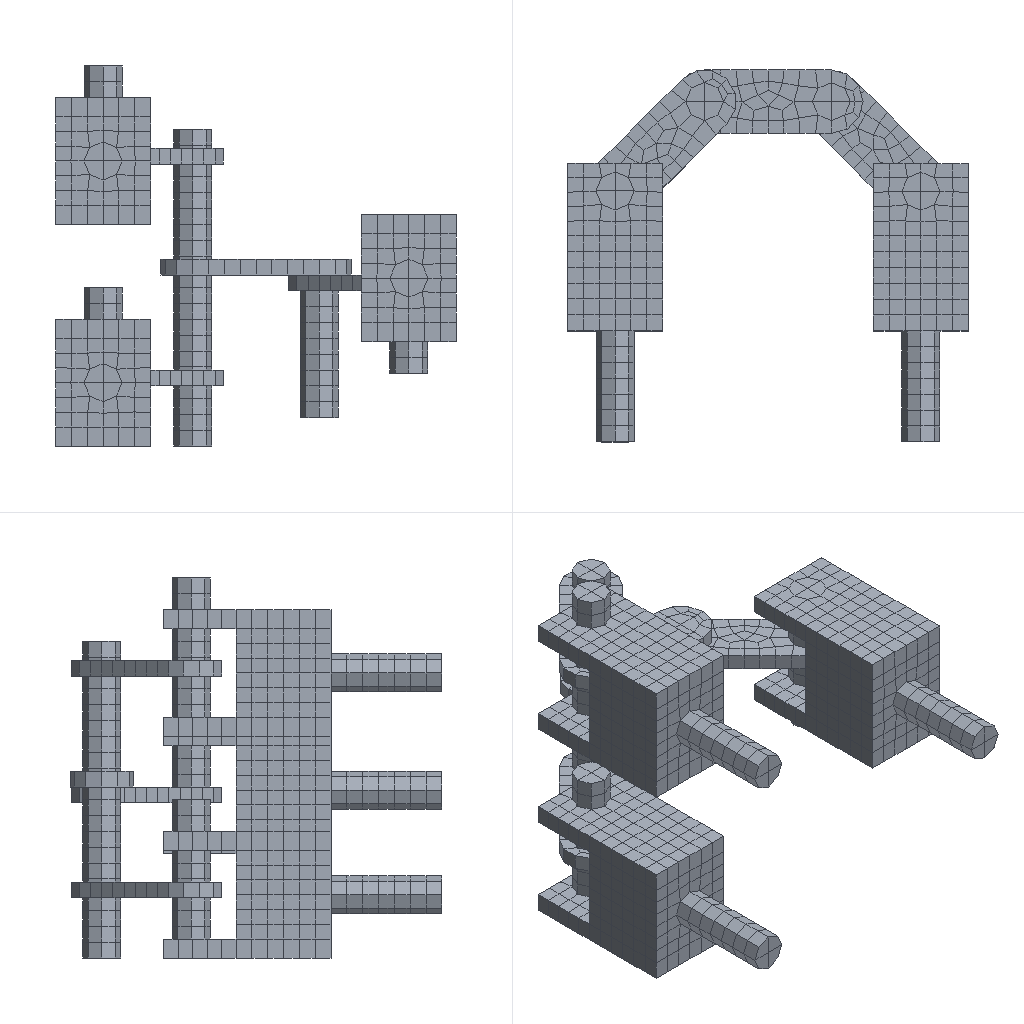Simulation study | abaqus
Set-up summary:
category,name,step,type,value,unit,region
solver,abaqus
solver,version,,,Abaqus/Explicit 2020
units,not stated in the deck,,not stated
analysis,deck,,transient,transient
load_step,Step-1,Step-1,transient
load_step,requested,,,1
mesh,nodes,,,3136
mesh,elements,,,1496
element_type,C3D8R,,solid,1496
load,load commands in deck,,count,1
bc,support commands in deck,,count,10
material,MATERIAL-1,,in results
check,setup vs results,,match,"per instance, exact: element labels, types and connectivity; labels of the nodes the elements use; coordinates of those nodes at SINGLE_PRECISION in 12 of 15 instance(s)"
Abaqus input file, long lists of numbers shortened:
*Heading
** Job name: Job-1 Model name: Model-1
** Generated by: Abaqus/CAE 2020
*Preprint, echo=NO, model=NO, history=NO, contact=NO
**
** PARTS
**
*Part, name=Part-1
*End Part
**
*Part, name=Part-2
*End Part
**
*Part, name=Part-3
*End Part
**
*Part, name=Part-4
*End Part
**
**
** ASSEMBLY
**
*Assembly, name=Assembly
**
*Instance, name=Part-1-1, part=Part-1
*Node
      1,          15.,          15.,           0.
      2,         -15.,          15.,           0.
** (568 more lines like these left out)
*Element, type=C3D8R
 1, 205,  46,  45, 200, 216,  57,  58, 211
 2, 204,  33,  32, 197, 215,  70,  71, 208
** (314 more lines like these left out)
*Nset, nset=Set-1, generate
   1,  570,    1
*Elset, elset=Set-1, generate
   1,  316,    1
** Section: Section-1
*Solid Section, elset=Set-1, material=Material-1
,
*End Instance
**
*Instance, name=Part-2-1, part=Part-2
          0.,         29.1,           0.
*Node
      1,   -4.243,   -4.243,           0.
      2,           0.,          -6.,           0.
** (97 more lines like these left out)
*Element, type=C3D8R
 1, 16, 15, 18, 17,  7,  6,  9,  8
 2, 18, 11, 10, 17,  9,  2,  1,  8
** (38 more lines like these left out)
*Nset, nset=Set-1, generate
  1,  99,   1
*Elset, elset=Set-1, generate
  1,  40,   1
** Section: Section-1
*Solid Section, elset=Set-1, material=Material-1
,
*End Instance
**
*Instance, name=Part-3-1, part=Part-3
26.87, 58.798,          19.
26.87, 58.798,          19., 26.87, 58.798, 18., 45.
*Node
      1,  -2.243,  -44.243,           0.
      2,           2.,         -46.,           0.
** (134 more lines like these left out)
*Element, type=C3D8R
 1,  66,  27,  28,  65, 134,  95,  96, 133
 2,  29,   3,  65,  28,  97,  71, 133,  96
** (45 more lines like these left out)
*Nset, nset=Set-1, generate
   1,  136,    1
*Elset, elset=Set-1, generate
  1,  47,   1
** Section: Section-1
*Solid Section, elset=Set-1, material=Material-1
,
*End Instance
**
*Instance, name=Part-2-2, part=Part-2
          0.,           0.,          20.
          0.,           0.,          20., 1.,           0.,          20., 90.
*Node
      1,   -4.243,   -4.243,           0.
      2,           0.,          -6.,           0.
** (97 more lines like these left out)
*Element, type=C3D8R
 1, 16, 15, 18, 17,  7,  6,  9,  8
 2, 18, 11, 10, 17,  9,  2,  1,  8
** (38 more lines like these left out)
*Nset, nset=Set-1, generate
  1,  99,   1
*Elset, elset=Set-1, generate
  1,  40,   1
** Section: Section-1
*Solid Section, elset=Set-1, material=Material-1
,
*End Instance
**
*Instance, name=Part-4-1, part=Part-4
28.284, 57.384,           0.
*Node
      1,   -4.243,   -4.243,           0.
      2,           0.,          -6.,           0.
** (187 more lines like these left out)
*Element, type=C3D8R
 1,  18,  17,  16,  15,   9,   8,   7,   6
 2,  18,  11,  10,  17,   9,   2,   1,   8
** (78 more lines like these left out)
*Nset, nset=Set-1, generate
   1,  189,    1
*Elset, elset=Set-1, generate
  1,  80,   1
** Section: Section-1
*Solid Section, elset=Set-1, material=Material-1
,
*End Instance
**
*Instance, name=Part-1-2, part=Part-1
          0.,           0.,          70.
*Node
      1,          15.,          15.,           0.
      2,         -15.,          15.,           0.
** (568 more lines like these left out)
*Element, type=C3D8R
 1, 205,  46,  45, 200, 216,  57,  58, 211
 2, 204,  33,  32, 197, 215,  70,  71, 208
** (314 more lines like these left out)
*Nset, nset=Set-1, generate
   1,  570,    1
*Elset, elset=Set-1, generate
   1,  316,    1
** Section: Section-1
*Solid Section, elset=Set-1, material=Material-1
,
*End Instance
**
*Instance, name=Part-2-3, part=Part-2
-5.50620154243842e-15,         29.1,         120.
-5.50620154243842e-15,         29.1,         120., 0.7071, 28.393,         120.,         180.
*Node
      1,   -4.243,   -4.243,           0.
      2,           0.,          -6.,           0.
** (97 more lines like these left out)
*Element, type=C3D8R
 1, 16, 15, 18, 17,  7,  6,  9,  8
 2, 18, 11, 10, 17,  9,  2,  1,  8
** (38 more lines like these left out)
*Nset, nset=Set-1, generate
  1,  99,   1
*Elset, elset=Set-1, generate
  1,  40,   1
** Section: Section-1
*Solid Section, elset=Set-1, material=Material-1
,
*End Instance
**
*Instance, name=Part-3-2, part=Part-3
26.87, 58.798,          89.
26.87, 58.798,          89., 26.87, 58.798, 88., 45.
*Node
      1,  -2.243,  -44.243,           0.
      2,           2.,         -46.,           0.
** (134 more lines like these left out)
*Element, type=C3D8R
 1,  66,  27,  28,  65, 134,  95,  96, 133
 2,  29,   3,  65,  28,  97,  71, 133,  96
** (45 more lines like these left out)
*Nset, nset=Set-1, generate
   1,  136,    1
*Elset, elset=Set-1, generate
  1,  47,   1
** Section: Section-1
*Solid Section, elset=Set-1, material=Material-1
,
*End Instance
**
*Instance, name=Part-2-4, part=Part-2
7.105427357601e-15,           0.,          90.
7.105427357601e-15,           0.,          90., 1.,           0.,          90., 90.
*Node
      1,   -4.243,   -4.243,           0.
      2,           0.,          -6.,           0.
** (97 more lines like these left out)
*Element, type=C3D8R
 1, 16, 15, 18, 17,  7,  6,  9,  8
 2, 18, 11, 10, 17,  9,  2,  1,  8
** (38 more lines like these left out)
*Nset, nset=Set-1, generate
  1,  99,   1
*Elset, elset=Set-1, generate
  1,  40,   1
** Section: Section-1
*Solid Section, elset=Set-1, material=Material-1
,
*End Instance
**
*Instance, name=Part-3-3, part=Part-3
28.284, 55.384,          54.
28.284, 55.384,          54., 28.284, 55.384, 55., 90.
*Node
      1,  -2.243,  -44.243,           0.
      2,           2.,         -46.,           0.
** (134 more lines like these left out)
*Element, type=C3D8R
 1,  66,  27,  28,  65, 134,  95,  96, 133
 2,  29,   3,  65,  28,  97,  71, 133,  96
** (45 more lines like these left out)
*Nset, nset=Set-1, generate
   1,  136,    1
*Elset, elset=Set-1, generate
  1,  47,   1
** Section: Section-1
*Solid Section, elset=Set-1, material=Material-1
,
*End Instance
**
*Instance, name=Part-2-5, part=Part-2
68.284, 57.384,           9.
*Node
      1,   -4.243,   -4.243,           0.
      2,           0.,          -6.,           0.
** (97 more lines like these left out)
*Element, type=C3D8R
 1, 16, 15, 18, 17,  7,  6,  9,  8
 2, 18, 11, 10, 17,  9,  2,  1,  8
** (38 more lines like these left out)
*Nset, nset=Set-1, generate
  1,  99,   1
*Elset, elset=Set-1, generate
  1,  40,   1
** Section: Section-1
*Solid Section, elset=Set-1, material=Material-1
,
*End Instance
**
*Instance, name=Part-3-4, part=Part-3
66.87, 55.97,          49.
66.87, 55.97,          49., 66.87, 55.97, 50., 45.
*Node
      1,  -2.243,  -44.243,           0.
      2,           2.,         -46.,           0.
** (134 more lines like these left out)
*Element, type=C3D8R
 1,  66,  27,  28,  65, 134,  95,  96, 133
 2,  29,   3,  65,  28,  97,  71, 133,  96
** (45 more lines like these left out)
*Nset, nset=Set-1, generate
   1,  136,    1
*Elset, elset=Set-1, generate
  1,  47,   1
** Section: Section-1
*Solid Section, elset=Set-1, material=Material-1
,
*End Instance
**
*Instance, name=Part-1-3, part=Part-1
96.569, -3.19744231092045e-14,          33.
*Node
      1,          15.,          15.,           0.
      2,         -15.,          15.,           0.
** (568 more lines like these left out)
*Element, type=C3D8R
 1, 205,  46,  45, 200, 216,  57,  58, 211
 2, 204,  33,  32, 197, 215,  70,  71, 208
** (314 more lines like these left out)
*Nset, nset=Set-1, generate
   1,  570,    1
*Elset, elset=Set-1, generate
   1,  316,    1
** Section: Section-1
*Solid Section, elset=Set-1, material=Material-1
,
*End Instance
**
*Instance, name=Part-2-6, part=Part-2
96.569,         29.1,          23.
*Node
      1,   -4.243,   -4.243,           0.
      2,           0.,          -6.,           0.
** (97 more lines like these left out)
*Element, type=C3D8R
 1, 16, 15, 18, 17,  7,  6,  9,  8
 2, 18, 11, 10, 17,  9,  2,  1,  8
** (38 more lines like these left out)
*Nset, nset=Set-1, generate
  1,  99,   1
*Elset, elset=Set-1, generate
  1,  40,   1
** Section: Section-1
*Solid Section, elset=Set-1, material=Material-1
,
*End Instance
**
*Instance, name=Part-2-7, part=Part-2
96.569,           0.,          53.
96.569,           0.,          53., 97.569,           0.,          53., 90.
*Node
      1,   -4.243,   -4.243,           0.
      2,           0.,          -6.,           0.
** (97 more lines like these left out)
*Element, type=C3D8R
 1, 16, 15, 18, 17,  7,  6,  9,  8
 2, 18, 11, 10, 17,  9,  2,  1,  8
** (38 more lines like these left out)
*Nset, nset=Set-1, generate
  1,  99,   1
*Elset, elset=Set-1, generate
  1,  40,   1
** Section: Section-1
*Solid Section, elset=Set-1, material=Material-1
,
*End Instance
**
*Node
      1, 7.10542736e-15,         -50.,          90.
*Node
      2, 3.67394029e-16,          15.,          90.
*Node
      3, 3.67394029e-16,          15.,          20.
*Node
      4,           0.,         -50.,          20.
*Node
      5,   96.569,         -50.,          53.
*Node
      6,   96.569,          15.,          53.
*Nset, nset=Set-13
 3, 4
*Nset, nset=Set-14
 4,
*Nset, nset=Set-15
 3, 4
*Nset, nset=Set-16, instance=Part-2-2, generate
 91,  99,   1
*Nset, nset=Set-16, instance=Part-2-4, generate
 91,  99,   1
*Nset, nset=Set-16
 1, 4, 5
*Nset, nset=Set-16, instance=Part-2-7, generate
 91,  99,   1
*Elset, elset=Set-16, instance=Part-2-2, generate
 37,  40,   1
*Elset, elset=Set-16, instance=Part-2-4, generate
 37,  40,   1
*Elset, elset=Set-16, instance=Part-2-7, generate
 37,  40,   1
*Nset, nset=Set-17, instance=Part-2-1, generate
 1,  9,  1
*Nset, nset=Set-17, instance=Part-2-3, generate
 91,  99,   1
*Nset, nset=Set-17, instance=Part-2-6, generate
 91,  99,   1
*Elset, elset=Set-17, instance=Part-2-1, generate
 1,  4,  1
*Elset, elset=Set-17, instance=Part-2-3, generate
 37,  40,   1
*Elset, elset=Set-17, instance=Part-2-6, generate
 37,  40,   1
*Nset, nset=Set-18, instance=Part-2-1
  1,  2,  3,  4,  5,  6,  7,  8,  9, 91, 92, 93, 94, 95, 96, 97
 98, 99
*Nset, nset=Set-18, instance=Part-4-1
   1,   2,   3,   4,   5,   6,   7,   8,   9, 181, 182, 183, 184, 185, 186, 187
 188, 189
*Nset, nset=Set-18, instance=Part-2-3
  1,  2,  3,  4,  5,  6,  7,  8,  9, 91, 92, 93, 94, 95, 96, 97
 98, 99
*Nset, nset=Set-18, instance=Part-2-5
  1,  2,  3,  4,  5,  6,  7,  8,  9, 91, 92, 93, 94, 95, 96, 97
 98, 99
*Nset, nset=Set-18, instance=Part-2-6
  1,  2,  3,  4,  5,  6,  7,  8,  9, 91, 92, 93, 94, 95, 96, 97
 98, 99
*Elset, elset=Set-18, instance=Part-2-1
  1,  2,  3,  4, 37, 38, 39, 40
*Elset, elset=Set-18, instance=Part-4-1
  1,  2,  3,  4, 77, 78, 79, 80
*Elset, elset=Set-18, instance=Part-2-3
  1,  2,  3,  4, 37, 38, 39, 40
*Elset, elset=Set-18, instance=Part-2-5
  1,  2,  3,  4, 37, 38, 39, 40
*Elset, elset=Set-18, instance=Part-2-6
  1,  2,  3,  4, 37, 38, 39, 40
*Nset, nset=Set-19, instance=Part-1-1
   7,  10,  18,  19,  21,  72,  73,  74,  75,  76, 113, 114, 115, 116, 117, 127
 128, 129, 130, 131, 132, 133, 134, 135, 136, 137, 138, 139, 140, 141, 142, 143
** (1 more lines like these left out)
*Nset, nset=Set-19, instance=Part-1-2
   7,  10,  18,  19,  21,  72,  73,  74,  75,  76, 113, 114, 115, 116, 117, 127
 128, 129, 130, 131, 132, 133, 134, 135, 136, 137, 138, 139, 140, 141, 142, 143
** (1 more lines like these left out)
*Elset, elset=Set-19, instance=Part-1-1, generate
 59,  90,   1
*Elset, elset=Set-19, instance=Part-1-2, generate
 59,  90,   1
*Nset, nset=Set-20, instance=Part-2-1
  1,  2,  3,  4,  5,  6,  7,  8,  9, 91, 92, 93, 94, 95, 96, 97
 98, 99
*Nset, nset=Set-20, instance=Part-3-1, generate
   1,  136,    1
*Nset, nset=Set-20, instance=Part-4-1
   1,   2,   3,   4,   5,   6,   7,   8,   9, 181, 182, 183, 184, 185, 186, 187
 188, 189
*Nset, nset=Set-20, instance=Part-2-3
  1,  2,  3,  4,  5,  6,  7,  8,  9, 91, 92, 93, 94, 95, 96, 97
 98, 99
*Nset, nset=Set-20, instance=Part-3-2, generate
   1,  136,    1
*Nset, nset=Set-20, instance=Part-2-5
  1,  2,  3,  4,  5,  6,  7,  8,  9, 91, 92, 93, 94, 95, 96, 97
 98, 99
*Nset, nset=Set-20, instance=Part-3-3, generate
   1,  136,    1
*Nset, nset=Set-20, instance=Part-3-4, generate
   1,  136,    1
*Nset, nset=Set-20, instance=Part-2-6
  1,  2,  3,  4,  5,  6,  7,  8,  9, 91, 92, 93, 94, 95, 96, 97
 98, 99
*Elset, elset=Set-20, instance=Part-2-1
  1,  2,  3,  4, 37, 38, 39, 40
*Elset, elset=Set-20, instance=Part-3-1, generate
  1,  47,   1
*Elset, elset=Set-20, instance=Part-4-1
  1,  2,  3,  4, 77, 78, 79, 80
*Elset, elset=Set-20, instance=Part-2-3
  1,  2,  3,  4, 37, 38, 39, 40
*Elset, elset=Set-20, instance=Part-3-2, generate
  1,  47,   1
*Elset, elset=Set-20, instance=Part-2-5
  1,  2,  3,  4, 37, 38, 39, 40
*Elset, elset=Set-20, instance=Part-3-3, generate
  1,  47,   1
*Elset, elset=Set-20, instance=Part-3-4, generate
  1,  47,   1
*Elset, elset=Set-20, instance=Part-2-6
  1,  2,  3,  4, 37, 38, 39, 40
*Nset, nset=Wire-1-Set-1
 3, 4
*Nset, nset=Wire-2-Set-1
 3, 4
*Nset, nset=b_Set-8, instance=Part-1-1, generate
   1,  570,    1
*Elset, elset=b_Set-8, instance=Part-1-1, generate
   1,  316,    1
*Nset, nset=b_Set-10, instance=Part-2-2, generate
  1,  99,   1
*Elset, elset=b_Set-10, instance=Part-2-2, generate
  1,  40,   1
*End Assembly
*Amplitude, name=Amp-1
             0.,              0.,          0.0005,              1.
**
** MATERIALS
**
*Material, name=Material-1
*Density
 7.85e-09,
*Elastic
210000., 0.3
**
** INTERACTION PROPERTIES
**
*Surface Interaction, name=IntProp-1
*Surface Behavior, pressure-overclosure=HARD
**
** CONTACT INITIALIZATION DATA
**
*Contact Initialization Data, name=CInit-1, INTERFERENCE FIT
**
** INTERACTIONS
**
** Interaction: Int-1
*Contact, op=NEW
*Contact Inclusions, ALL EXTERIOR
*Contact Property Assignment
 ,  , IntProp-1
** ----------------------------------------------------------------
**
** STEP: Step-1
**
*Step, name=Step-1, nlgeom=YES
*Dynamic, Explicit
, 0.0005
*Bulk Viscosity
0.06, 1.2
**
** BOUNDARY CONDITIONS
**
** Name: BC-1 Type: 对称/反对称/完全固定
*Boundary
Set-16, ENCASTRE
** Name: BC-2 Type: 位移/转角
*Boundary
Set-20, 3, 3
Set-20, 4, 4
Set-20, 5, 5
** Name: BC-3 Type: 位移/转角
*Boundary, amplitude=Amp-1
Set-19, 1, 1
Set-19, 2, 2, -20.
Set-19, 3, 3
Set-19, 4, 4
Set-19, 5, 5
Set-19, 6, 6
**
** OUTPUT REQUESTS
**
*Restart, write, number interval=1, time marks=NO
**
** FIELD OUTPUT: F-Output-1
**
*Output, field, number interval=50
*Node Output
CF, RF, U, V
*Element Output, directions=YES
E, LE, MISES, MISESMAX, PE, PEEQ, PEMAG, S
*Contact Output
CDISP, CSTRESS
**
** HISTORY OUTPUT: H-Output-1
**
*Output, history, variable=PRESELECT, frequency=1
*End Step
Results summary:
result,step,Step-1,completed,increments=1808 time=0.0005/0.0005
result,analysis,,,transient
result,last_loadstep,,,1
result,primary field,,,U
result,reaction total,,FX,-49491.709,model units
result,reaction total,,FY,-99667.236,model units
result,reaction total,,FZ,-49605.941,model units